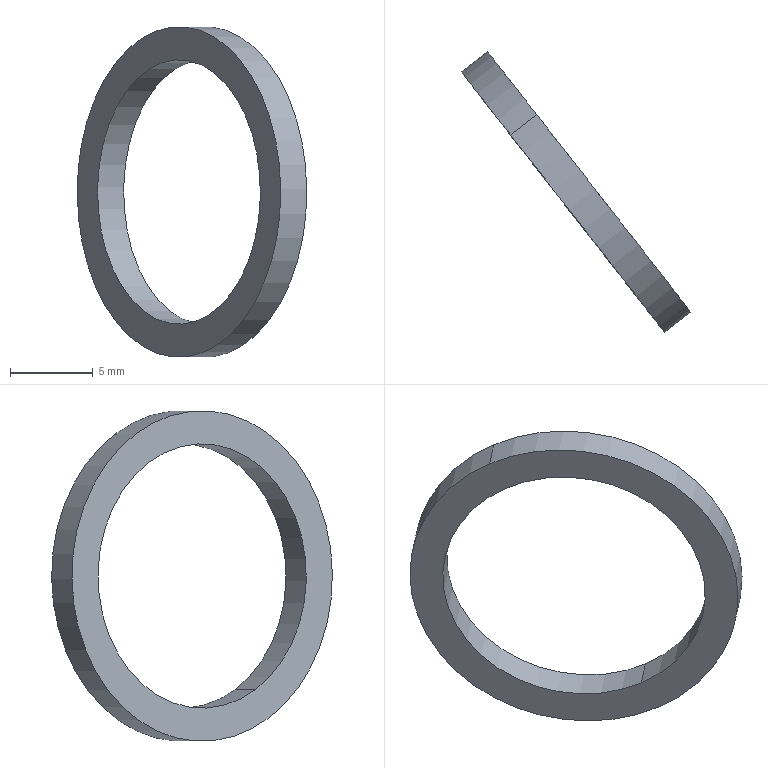Part | SolidWorks | features BaseBody 1 | 1 solid | 6 faces | box 13.889 x 16.992 x 20 mm | volume 226.195 mm3 | cylinder 4 | plane 2 | commonest cylinder face diameters 16 x2 20 x2
STEP:
#1=CARTESIAN_POINT('',(2.011,101.417,78.83));
#2=VERTEX_POINT('',#1);
#3=CARTESIAN_POINT('',(8.335,93.323,61.67));
#4=VERTEX_POINT('',#3);
#5=CARTESIAN_POINT('',(5.173,97.37,70.25));
#6=DIRECTION('',(0.788,0.6157,0.));
#7=DIRECTION('',(-0.3162,0.4047,0.858));
#8=AXIS2_PLACEMENT_3D('',#5,#6,#7);
#9=CIRCLE('',#8,10.);
#10=EDGE_CURVE('',#2,#4,#9,.T.);
#11=ORIENTED_EDGE('',*,*,#10,.F.);
#12=CARTESIAN_POINT('',(0.4353,100.186,78.83));
#13=VERTEX_POINT('',#12);
#14=CARTESIAN_POINT('',(2.011,101.417,78.83));
#15=DIRECTION('',(-0.788,-0.6157,0.));
#16=VECTOR('',#15,1000.);
#17=LINE('',#14,#16);
#18=EDGE_CURVE('',#2,#13,#17,.T.);
#19=ORIENTED_EDGE('',*,*,#18,.T.);
#20=CARTESIAN_POINT('',(6.759,92.092,61.67));
#21=VERTEX_POINT('',#20);
#22=CARTESIAN_POINT('',(3.597,96.139,70.25));
#23=DIRECTION('',(0.788,0.6157,0.));
#24=DIRECTION('',(-0.3162,0.4047,0.858));
#25=AXIS2_PLACEMENT_3D('',#22,#23,#24);
#26=CIRCLE('',#25,10.);
#27=EDGE_CURVE('',#13,#21,#26,.T.);
#28=ORIENTED_EDGE('',*,*,#27,.T.);
#29=CARTESIAN_POINT('',(8.335,93.323,61.67));
#30=DIRECTION('',(-0.788,-0.6157,0.));
#31=VECTOR('',#30,1000.);
#32=LINE('',#29,#31);
#33=EDGE_CURVE('',#4,#21,#32,.T.);
#34=ORIENTED_EDGE('',*,*,#33,.F.);
#35=EDGE_LOOP('',(#11,#19,#28,#34));
#36=FACE_OUTER_BOUND('',#35,.T.);
#37=CARTESIAN_POINT('',(5.173,97.37,70.25));
#38=DIRECTION('',(-0.788,-0.6157,0.));
#39=DIRECTION('',(0.3162,-0.4047,-0.858));
#40=AXIS2_PLACEMENT_3D('',#37,#38,#39);
#41=CYLINDRICAL_SURFACE('',#40,10.);
#42=ADVANCED_FACE('',(#36),#41,.T.);
#43=CARTESIAN_POINT('',(7.703,94.132,63.386));
#44=VERTEX_POINT('',#43);
#45=CARTESIAN_POINT('',(2.644,100.608,77.114));
#46=VERTEX_POINT('',#45);
#47=CARTESIAN_POINT('',(5.173,97.37,70.25));
#48=DIRECTION('',(0.788,0.6157,0.));
#49=DIRECTION('',(-0.3162,0.4047,0.858));
#50=AXIS2_PLACEMENT_3D('',#47,#48,#49);
#51=CIRCLE('',#50,8.);
#52=EDGE_CURVE('',#44,#46,#51,.T.);
#53=ORIENTED_EDGE('',*,*,#52,.T.);
#54=CARTESIAN_POINT('',(1.068,99.377,77.114));
#55=VERTEX_POINT('',#54);
#56=CARTESIAN_POINT('',(2.644,100.608,77.114));
#57=DIRECTION('',(-0.788,-0.6157,0.));
#58=VECTOR('',#57,1000.);
#59=LINE('',#56,#58);
#60=EDGE_CURVE('',#46,#55,#59,.T.);
#61=ORIENTED_EDGE('',*,*,#60,.T.);
#62=CARTESIAN_POINT('',(6.127,92.901,63.386));
#63=VERTEX_POINT('',#62);
#64=CARTESIAN_POINT('',(3.597,96.139,70.25));
#65=DIRECTION('',(0.788,0.6157,0.));
#66=DIRECTION('',(-0.3162,0.4047,0.858));
#67=AXIS2_PLACEMENT_3D('',#64,#65,#66);
#68=CIRCLE('',#67,8.);
#69=EDGE_CURVE('',#63,#55,#68,.T.);
#70=ORIENTED_EDGE('',*,*,#69,.F.);
#71=CARTESIAN_POINT('',(7.703,94.132,63.386));
#72=DIRECTION('',(-0.788,-0.6157,0.));
#73=VECTOR('',#72,1000.);
#74=LINE('',#71,#73);
#75=EDGE_CURVE('',#44,#63,#74,.T.);
#76=ORIENTED_EDGE('',*,*,#75,.F.);
#77=EDGE_LOOP('',(#53,#61,#70,#76));
#78=FACE_OUTER_BOUND('',#77,.T.);
#79=CARTESIAN_POINT('',(5.173,97.37,70.25));
#80=DIRECTION('',(-0.788,-0.6157,0.));
#81=DIRECTION('',(0.3162,-0.4047,-0.858));
#82=AXIS2_PLACEMENT_3D('',#79,#80,#81);
#83=CYLINDRICAL_SURFACE('',#82,8.);
#84=ADVANCED_FACE('',(#78),#83,.F.);
#85=CARTESIAN_POINT('',(3.597,96.139,70.25));
#86=DIRECTION('',(0.788,0.6157,0.));
#87=DIRECTION('',(-0.3162,0.4047,0.858));
#88=AXIS2_PLACEMENT_3D('',#85,#86,#87);
#89=CIRCLE('',#88,10.);
#90=EDGE_CURVE('',#21,#13,#89,.T.);
#91=ORIENTED_EDGE('',*,*,#90,.F.);
#92=ORIENTED_EDGE('',*,*,#27,.F.);
#93=EDGE_LOOP('',(#91,#92));
#94=FACE_OUTER_BOUND('',#93,.T.);
#95=ORIENTED_EDGE('',*,*,#69,.T.);
#96=CARTESIAN_POINT('',(3.597,96.139,70.25));
#97=DIRECTION('',(0.788,0.6157,0.));
#98=DIRECTION('',(-0.3162,0.4047,0.858));
#99=AXIS2_PLACEMENT_3D('',#96,#97,#98);
#100=CIRCLE('',#99,8.);
#101=EDGE_CURVE('',#55,#63,#100,.T.);
#102=ORIENTED_EDGE('',*,*,#101,.T.);
#103=EDGE_LOOP('',(#95,#102));
#104=FACE_BOUND('',#103,.T.);
#105=CARTESIAN_POINT('',(3.597,96.139,70.25));
#106=DIRECTION('',(0.788,0.6157,0.));
#107=DIRECTION('',(0.,0.,-1.));
#108=AXIS2_PLACEMENT_3D('',#105,#106,#107);
#109=PLANE('',#108);
#110=ADVANCED_FACE('',(#94,#104),#109,.F.);
#111=ORIENTED_EDGE('',*,*,#60,.F.);
#112=CARTESIAN_POINT('',(5.173,97.37,70.25));
#113=DIRECTION('',(0.788,0.6157,0.));
#114=DIRECTION('',(-0.3162,0.4047,0.858));
#115=AXIS2_PLACEMENT_3D('',#112,#113,#114);
#116=CIRCLE('',#115,8.);
#117=EDGE_CURVE('',#46,#44,#116,.T.);
#118=ORIENTED_EDGE('',*,*,#117,.T.);
#119=ORIENTED_EDGE('',*,*,#75,.T.);
#120=ORIENTED_EDGE('',*,*,#101,.F.);
#121=EDGE_LOOP('',(#111,#118,#119,#120));
#122=FACE_OUTER_BOUND('',#121,.T.);
#123=CARTESIAN_POINT('',(5.173,97.37,70.25));
#124=DIRECTION('',(-0.788,-0.6157,0.));
#125=DIRECTION('',(0.3162,-0.4047,-0.858));
#126=AXIS2_PLACEMENT_3D('',#123,#124,#125);
#127=CYLINDRICAL_SURFACE('',#126,8.);
#128=ADVANCED_FACE('',(#122),#127,.F.);
#129=ORIENTED_EDGE('',*,*,#18,.F.);
#130=CARTESIAN_POINT('',(5.173,97.37,70.25));
#131=DIRECTION('',(0.788,0.6157,0.));
#132=DIRECTION('',(-0.3162,0.4047,0.858));
#133=AXIS2_PLACEMENT_3D('',#130,#131,#132);
#134=CIRCLE('',#133,10.);
#135=EDGE_CURVE('',#4,#2,#134,.T.);
#136=ORIENTED_EDGE('',*,*,#135,.F.);
#137=ORIENTED_EDGE('',*,*,#33,.T.);
#138=ORIENTED_EDGE('',*,*,#90,.T.);
#139=EDGE_LOOP('',(#129,#136,#137,#138));
#140=FACE_OUTER_BOUND('',#139,.T.);
#141=CARTESIAN_POINT('',(5.173,97.37,70.25));
#142=DIRECTION('',(-0.788,-0.6157,0.));
#143=DIRECTION('',(0.3162,-0.4047,-0.858));
#144=AXIS2_PLACEMENT_3D('',#141,#142,#143);
#145=CYLINDRICAL_SURFACE('',#144,10.);
#146=ADVANCED_FACE('',(#140),#145,.T.);
#147=ORIENTED_EDGE('',*,*,#52,.F.);
#148=ORIENTED_EDGE('',*,*,#117,.F.);
#149=EDGE_LOOP('',(#147,#148));
#150=FACE_BOUND('',#149,.T.);
#151=ORIENTED_EDGE('',*,*,#135,.T.);
#152=ORIENTED_EDGE('',*,*,#10,.T.);
#153=EDGE_LOOP('',(#151,#152));
#154=FACE_OUTER_BOUND('',#153,.T.);
#155=CARTESIAN_POINT('',(5.173,97.37,70.25));
#156=DIRECTION('',(0.788,0.6157,0.));
#157=DIRECTION('',(0.,0.,-1.));
#158=AXIS2_PLACEMENT_3D('',#155,#156,#157);
#159=PLANE('',#158);
#160=ADVANCED_FACE('',(#150,#154),#159,.T.);
#161=CLOSED_SHELL('',(#42,#84,#110,#128,#146,#160));
#162=MANIFOLD_SOLID_BREP('',#161);
#163=CARTESIAN_POINT('',(0.,0.,0.));
#164=DIRECTION('',(0.,0.,1.));
#165=DIRECTION('',(1.,0.,0.));
#166=AXIS2_PLACEMENT_3D('',#163,#164,#165);
#167=(LENGTH_UNIT()NAMED_UNIT(*)SI_UNIT(.MILLI.,.METRE.));
#168=UNCERTAINTY_MEASURE_WITH_UNIT(LENGTH_MEASURE(0.00001),#167,'','');
#169=(NAMED_UNIT(*)PLANE_ANGLE_UNIT()SI_UNIT($,.RADIAN.));
#170=(NAMED_UNIT(*)SI_UNIT($,.STERADIAN.)SOLID_ANGLE_UNIT());
#171=(GEOMETRIC_REPRESENTATION_CONTEXT(3)GLOBAL_UNCERTAINTY_ASSIGNED_CONTEXT((#168))GLOBAL_UNIT_ASSIGNED_CONTEXT((#167,#169,#170))REPRESENTATION_CONTEXT('',''));
#172=ADVANCED_BREP_SHAPE_REPRESENTATION('',(#162,#166),#171);